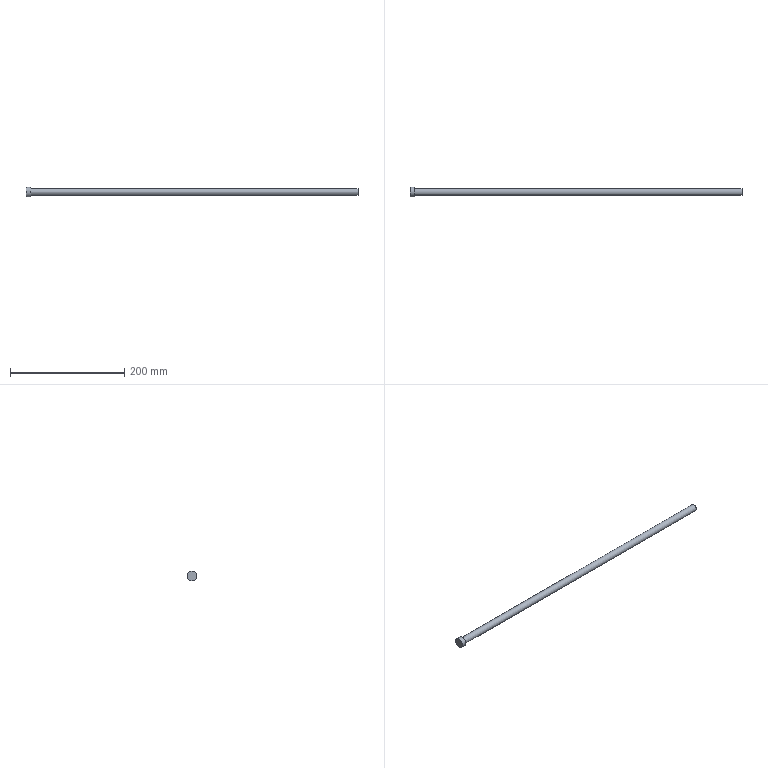Part | STEP file | solid 11 | 1 solid | 5 faces | box 580 x 17 x 17 mm | volume 66508 mm3 | plane 3 | cylinder 2 | commonest cylinder face diameters 12 x1 17 x1